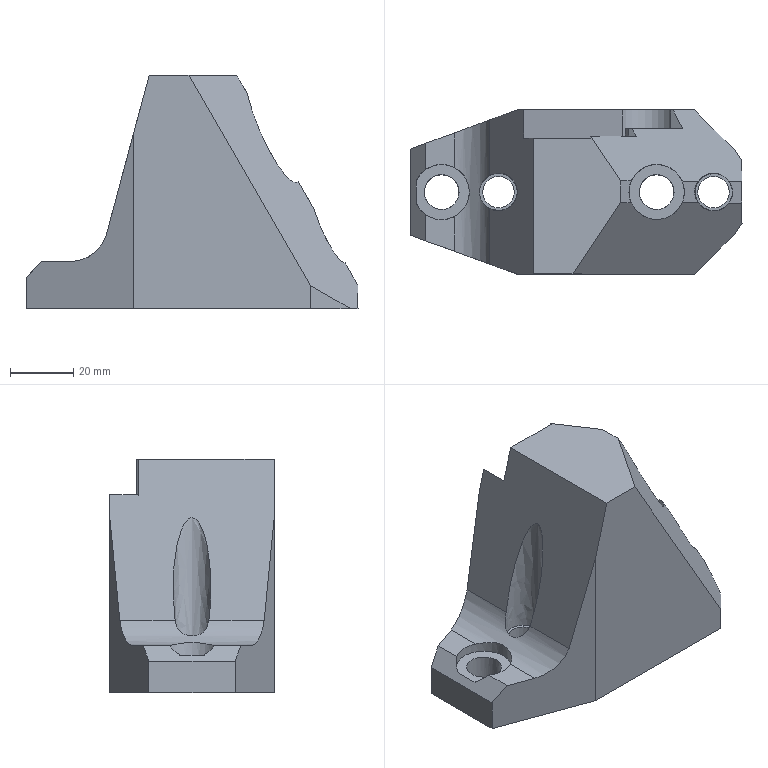Part | NX | features solid 2 | 1 solid | 41 faces | box 105 x 52 x 74 mm | volume 179080 mm3 | plane 30 | cylinder 8 | spline 3 | commonest cylinder face diameters 10 x2 11 x2 17.5 x1 17.501 x1 18.3 x1 24 x1
STEP:
#1=CARTESIAN_POINT('',(-407.032,-240.,159.));
#2=VERTEX_POINT('',#1);
#3=CARTESIAN_POINT('',(-407.032,-197.,159.));
#4=VERTEX_POINT('',#3);
#5=CARTESIAN_POINT('',(-407.032,-280.,159.));
#6=DIRECTION('',(0.,1.,0.));
#7=VECTOR('',#6,1000.);
#8=LINE('',#5,#7);
#9=EDGE_CURVE('',#2,#4,#8,.T.);
#10=ORIENTED_EDGE('',*,*,#9,.F.);
#11=CARTESIAN_POINT('',(-394.445,-240.,159.));
#12=VERTEX_POINT('',#11);
#13=CARTESIAN_POINT('',(-436.383,-240.,159.));
#14=DIRECTION('',(1.,0.,0.));
#15=VECTOR('',#14,1000.);
#16=LINE('',#13,#15);
#17=EDGE_CURVE('',#2,#12,#16,.T.);
#18=ORIENTED_EDGE('',*,*,#17,.T.);
#19=CARTESIAN_POINT('',(-379.421,-217.464,159.));
#20=VERTEX_POINT('',#19);
#21=CARTESIAN_POINT('',(-399.355,-247.365,159.));
#22=DIRECTION('',(0.5547,0.8321,0.));
#23=VECTOR('',#22,1000.);
#24=LINE('',#21,#23);
#25=EDGE_CURVE('',#12,#20,#24,.T.);
#26=ORIENTED_EDGE('',*,*,#25,.T.);
#27=CARTESIAN_POINT('',(-379.421,-210.536,159.));
#28=VERTEX_POINT('',#27);
#29=CARTESIAN_POINT('',(-379.421,-217.464,159.));
#30=DIRECTION('',(0.,1.,0.));
#31=VECTOR('',#30,1000.);
#32=LINE('',#29,#31);
#33=EDGE_CURVE('',#20,#28,#32,.T.);
#34=ORIENTED_EDGE('',*,*,#33,.T.);
#35=CARTESIAN_POINT('',(-388.839,-196.41,159.));
#36=VERTEX_POINT('',#35);
#37=CARTESIAN_POINT('',(-385.487,-201.438,159.));
#38=DIRECTION('',(-0.5547,0.8321,0.));
#39=VECTOR('',#38,1000.);
#40=LINE('',#37,#39);
#41=EDGE_CURVE('',#28,#36,#40,.T.);
#42=ORIENTED_EDGE('',*,*,#41,.T.);
#43=CARTESIAN_POINT('',(-388.839,-197.,159.));
#44=VERTEX_POINT('',#43);
#45=CARTESIAN_POINT('',(-388.839,-240.,159.));
#46=DIRECTION('',(0.,-1.,0.));
#47=VECTOR('',#46,1000.);
#48=LINE('',#45,#47);
#49=EDGE_CURVE('',#36,#44,#48,.T.);
#50=ORIENTED_EDGE('',*,*,#49,.T.);
#51=CARTESIAN_POINT('',(-407.032,-197.,159.));
#52=DIRECTION('',(-1.,0.,0.));
#53=VECTOR('',#52,1000.);
#54=LINE('',#51,#53);
#55=EDGE_CURVE('',#44,#4,#54,.T.);
#56=ORIENTED_EDGE('',*,*,#55,.T.);
#57=EDGE_LOOP('',(#10,#18,#26,#34,#42,#50,#56));
#58=FACE_BOUND('',#57,.T.);
#59=CARTESIAN_POINT('',(-407.032,-240.,159.));
#60=DIRECTION('',(0.,0.,1.));
#61=DIRECTION('',(0.,-1.,0.));
#62=AXIS2_PLACEMENT_3D('',#59,#60,#61);
#63=PLANE('',#62);
#64=ADVANCED_FACE('',(#58),#63,.T.);
#65=CARTESIAN_POINT('',(-432.,-195.279,100.002));
#66=VERTEX_POINT('',#65);
#67=CARTESIAN_POINT('',(-420.73,-191.177,107.88));
#68=VERTEX_POINT('',#67);
#69=CARTESIAN_POINT('',(-432.,-195.279,112.002));
#70=DIRECTION('',(0.342,-0.9397,0.));
#71=DIRECTION('',(0.9397,0.342,0.));
#72=AXIS2_PLACEMENT_3D('',#69,#70,#71);
#73=ELLIPSE('',#72,12.77,12.);
#74=EDGE_CURVE('',#66,#68,#73,.T.);
#75=ORIENTED_EDGE('',*,*,#74,.F.);
#76=CARTESIAN_POINT('',(-432.,-206.218,100.002));
#77=VERTEX_POINT('',#76);
#78=CARTESIAN_POINT('',(-432.,-280.,100.002));
#79=DIRECTION('',(0.,1.,0.));
#80=VECTOR('',#79,1000.);
#81=LINE('',#78,#80);
#82=EDGE_CURVE('',#77,#66,#81,.T.);
#83=ORIENTED_EDGE('',*,*,#82,.F.);
#84=CARTESIAN_POINT('',(-432.,-221.782,100.002));
#85=VERTEX_POINT('',#84);
#86=CARTESIAN_POINT('',(-432.,-206.218,100.002));
#87=CARTESIAN_POINT('',(-430.573,-206.951,100.002));
#88=CARTESIAN_POINT('',(-428.146,-209.212,100.538));
#89=CARTESIAN_POINT('',(-426.801,-214.004,101.205));
#90=CARTESIAN_POINT('',(-428.15,-218.796,100.536));
#91=CARTESIAN_POINT('',(-430.581,-221.053,100.002));
#92=CARTESIAN_POINT('',(-432.,-221.782,100.002));
#93=B_SPLINE_CURVE_WITH_KNOTS('',3,(#86,#87,#88,#89,#90,#91,#92),.UNSPECIFIED.,.F.,.F.,(4,1,1,1,4),(0.059,0.06377,0.06854,0.07331,0.07807),.UNSPECIFIED.);
#94=EDGE_CURVE('',#77,#85,#93,.T.);
#95=ORIENTED_EDGE('',*,*,#94,.T.);
#96=CARTESIAN_POINT('',(-432.,-232.721,100.002));
#97=VERTEX_POINT('',#96);
#98=CARTESIAN_POINT('',(-432.,-280.,100.002));
#99=DIRECTION('',(0.,1.,0.));
#100=VECTOR('',#99,1000.);
#101=LINE('',#98,#100);
#102=EDGE_CURVE('',#97,#85,#101,.T.);
#103=ORIENTED_EDGE('',*,*,#102,.F.);
#104=CARTESIAN_POINT('',(-420.73,-236.823,107.88));
#105=VERTEX_POINT('',#104);
#106=CARTESIAN_POINT('',(-432.,-232.721,112.002));
#107=DIRECTION('',(-0.342,-0.9397,0.));
#108=DIRECTION('',(-0.9397,0.342,0.));
#109=AXIS2_PLACEMENT_3D('',#106,#107,#108);
#110=ELLIPSE('',#109,12.77,12.);
#111=EDGE_CURVE('',#97,#105,#110,.T.);
#112=ORIENTED_EDGE('',*,*,#111,.T.);
#113=CARTESIAN_POINT('',(-420.73,-219.34,107.88));
#114=VERTEX_POINT('',#113);
#115=CARTESIAN_POINT('',(-420.73,-280.,107.88));
#116=DIRECTION('',(0.,1.,0.));
#117=VECTOR('',#116,1000.);
#118=LINE('',#115,#117);
#119=EDGE_CURVE('',#105,#114,#118,.T.);
#120=ORIENTED_EDGE('',*,*,#119,.T.);
#121=CARTESIAN_POINT('',(-420.73,-208.66,107.88));
#122=VERTEX_POINT('',#121);
#123=CARTESIAN_POINT('',(-420.73,-219.34,107.88));
#124=CARTESIAN_POINT('',(-420.975,-219.215,107.209));
#125=CARTESIAN_POINT('',(-421.568,-218.877,105.953));
#126=CARTESIAN_POINT('',(-422.701,-217.863,104.349));
#127=CARTESIAN_POINT('',(-423.711,-216.191,103.305));
#128=CARTESIAN_POINT('',(-424.14,-214.019,102.937));
#129=CARTESIAN_POINT('',(-423.728,-211.846,103.291));
#130=CARTESIAN_POINT('',(-422.369,-209.586,104.684));
#131=CARTESIAN_POINT('',(-421.223,-208.911,106.533));
#132=CARTESIAN_POINT('',(-420.73,-208.66,107.88));
#133=B_SPLINE_CURVE_WITH_KNOTS('',3,(#123,#124,#125,#126,#127,#128,#129,#130,#131,#132),.UNSPECIFIED.,.F.,.F.,(4,1,1,1,1,1,1,4),(0.,0.002143,0.004286,0.006429,0.008572,0.01071,0.01286,0.01714),.UNSPECIFIED.);
#134=EDGE_CURVE('',#114,#122,#133,.T.);
#135=ORIENTED_EDGE('',*,*,#134,.T.);
#136=CARTESIAN_POINT('',(-420.73,-280.,107.88));
#137=DIRECTION('',(0.,1.,0.));
#138=VECTOR('',#137,1000.);
#139=LINE('',#136,#138);
#140=EDGE_CURVE('',#122,#68,#139,.T.);
#141=ORIENTED_EDGE('',*,*,#140,.T.);
#142=EDGE_LOOP('',(#75,#83,#95,#103,#112,#120,#135,#141));
#143=FACE_BOUND('',#142,.T.);
#144=CARTESIAN_POINT('',(-432.,-280.,112.002));
#145=DIRECTION('',(0.,1.,0.));
#146=DIRECTION('',(0.,0.,1.));
#147=AXIS2_PLACEMENT_3D('',#144,#145,#146);
#148=CYLINDRICAL_SURFACE('',#147,12.);
#149=ADVANCED_FACE('',(#143),#148,.F.);
#150=CARTESIAN_POINT('',(-412.,-240.,140.46));
#151=VERTEX_POINT('',#150);
#152=CARTESIAN_POINT('',(-420.73,-240.,107.88));
#153=DIRECTION('',(-0.2588,0.,-0.9659));
#154=VECTOR('',#153,1000.);
#155=LINE('',#152,#154);
#156=EDGE_CURVE('',#2,#151,#155,.T.);
#157=ORIENTED_EDGE('',*,*,#156,.F.);
#158=ORIENTED_EDGE('',*,*,#9,.T.);
#159=CARTESIAN_POINT('',(-410.05,-197.,147.738));
#160=VERTEX_POINT('',#159);
#161=CARTESIAN_POINT('',(-420.73,-197.,107.88));
#162=DIRECTION('',(-0.2588,0.,-0.9659));
#163=VECTOR('',#162,1000.);
#164=LINE('',#161,#163);
#165=EDGE_CURVE('',#4,#160,#164,.T.);
#166=ORIENTED_EDGE('',*,*,#165,.T.);
#167=CARTESIAN_POINT('',(-410.05,-188.,147.738));
#168=VERTEX_POINT('',#167);
#169=CARTESIAN_POINT('',(-410.05,-197.,147.738));
#170=DIRECTION('',(0.,1.,0.));
#171=VECTOR('',#170,1000.);
#172=LINE('',#169,#171);
#173=EDGE_CURVE('',#168,#160,#172,.F.);
#174=ORIENTED_EDGE('',*,*,#173,.F.);
#175=CARTESIAN_POINT('',(-412.,-188.,140.46));
#176=VERTEX_POINT('',#175);
#177=CARTESIAN_POINT('',(-405.839,-188.,163.453));
#178=DIRECTION('',(0.2588,0.,0.9659));
#179=VECTOR('',#178,1000.);
#180=LINE('',#177,#179);
#181=EDGE_CURVE('',#176,#168,#180,.T.);
#182=ORIENTED_EDGE('',*,*,#181,.F.);
#183=CARTESIAN_POINT('',(-422.876,-191.959,99.869));
#184=DIRECTION('',(0.2577,0.09379,0.9617));
#185=VECTOR('',#184,1000.);
#186=LINE('',#183,#185);
#187=EDGE_CURVE('',#68,#176,#186,.T.);
#188=ORIENTED_EDGE('',*,*,#187,.F.);
#189=ORIENTED_EDGE('',*,*,#140,.F.);
#190=CARTESIAN_POINT('',(-420.73,-208.66,107.88));
#191=CARTESIAN_POINT('',(-419.967,-208.271,110.728));
#192=CARTESIAN_POINT('',(-418.819,-207.971,115.011));
#193=CARTESIAN_POINT('',(-417.281,-208.006,120.753));
#194=CARTESIAN_POINT('',(-416.131,-208.26,125.044));
#195=CARTESIAN_POINT('',(-414.988,-208.761,129.31));
#196=CARTESIAN_POINT('',(-414.04,-209.44,132.847));
#197=CARTESIAN_POINT('',(-413.301,-210.236,135.606));
#198=CARTESIAN_POINT('',(-412.759,-211.025,137.629));
#199=CARTESIAN_POINT('',(-412.336,-211.93,139.206));
#200=CARTESIAN_POINT('',(-412.057,-212.997,140.246));
#201=CARTESIAN_POINT('',(-411.963,-214.131,140.599));
#202=CARTESIAN_POINT('',(-412.098,-215.198,140.093));
#203=CARTESIAN_POINT('',(-412.388,-216.199,139.013));
#204=CARTESIAN_POINT('',(-412.817,-217.072,137.413));
#205=CARTESIAN_POINT('',(-413.355,-217.83,135.403));
#206=CARTESIAN_POINT('',(-414.098,-218.608,132.63));
#207=CARTESIAN_POINT('',(-415.032,-219.262,129.145));
#208=CARTESIAN_POINT('',(-416.164,-219.75,124.92));
#209=CARTESIAN_POINT('',(-417.303,-219.996,120.67));
#210=CARTESIAN_POINT('',(-418.832,-220.026,114.964));
#211=CARTESIAN_POINT('',(-419.972,-219.726,110.708));
#212=CARTESIAN_POINT('',(-420.73,-219.34,107.88));
#213=B_SPLINE_CURVE_WITH_KNOTS('',3,(#190,#191,#192,#193,#194,#195,#196,#197,#198,#199,#200,#201,#202,#203,#204,#205,#206,#207,#208,#209,#210,#211,#212),.UNSPECIFIED.,.F.,.F.,(4,1,1,1,1,1,1,1,1,1,1,1,1,1,1,1,1,1,1,1,4),(0.,0.008893,0.01334,0.01779,0.02223,0.02668,0.0289,0.03112,0.03335,0.03446,0.03557,0.03668,0.03779,0.04002,0.04224,0.04446,0.04891,0.05336,0.0578,0.06225,0.07114),.UNSPECIFIED.);
#214=EDGE_CURVE('',#122,#114,#213,.T.);
#215=ORIENTED_EDGE('',*,*,#214,.T.);
#216=ORIENTED_EDGE('',*,*,#119,.F.);
#217=CARTESIAN_POINT('',(-419.686,-237.202,111.774));
#218=DIRECTION('',(0.2577,-0.09379,0.9617));
#219=VECTOR('',#218,1000.);
#220=LINE('',#217,#219);
#221=EDGE_CURVE('',#105,#151,#220,.T.);
#222=ORIENTED_EDGE('',*,*,#221,.T.);
#223=EDGE_LOOP('',(#157,#158,#166,#174,#182,#188,#189,#215,#216,#222));
#224=FACE_BOUND('',#223,.T.);
#225=CARTESIAN_POINT('',(-420.73,-280.,107.88));
#226=DIRECTION('',(-0.9659,0.,0.2588));
#227=DIRECTION('',(0.2588,0.,0.9659));
#228=AXIS2_PLACEMENT_3D('',#225,#226,#227);
#229=PLANE('',#228);
#230=ADVANCED_FACE('',(#224),#229,.T.);
#231=CARTESIAN_POINT('',(-441.001,-229.445,100.002));
#232=VERTEX_POINT('',#231);
#233=CARTESIAN_POINT('',(-441.001,-221.181,100.002));
#234=VERTEX_POINT('',#233);
#235=CARTESIAN_POINT('',(-441.001,-280.,100.002));
#236=DIRECTION('',(0.,1.,0.));
#237=VECTOR('',#236,1000.);
#238=LINE('',#235,#237);
#239=EDGE_CURVE('',#232,#234,#238,.T.);
#240=ORIENTED_EDGE('',*,*,#239,.F.);
#241=CARTESIAN_POINT('',(-424.752,-235.359,100.002));
#242=DIRECTION('',(0.9397,-0.342,0.));
#243=VECTOR('',#242,1000.);
#244=LINE('',#241,#243);
#245=EDGE_CURVE('',#232,#97,#244,.T.);
#246=ORIENTED_EDGE('',*,*,#245,.T.);
#247=ORIENTED_EDGE('',*,*,#102,.T.);
#248=CARTESIAN_POINT('',(-436.,-214.,100.002));
#249=DIRECTION('',(0.,0.,1.));
#250=DIRECTION('',(1.,0.,0.));
#251=AXIS2_PLACEMENT_3D('',#248,#249,#250);
#252=CIRCLE('',#251,8.75);
#253=EDGE_CURVE('',#85,#234,#252,.F.);
#254=ORIENTED_EDGE('',*,*,#253,.T.);
#255=EDGE_LOOP('',(#240,#246,#247,#254));
#256=FACE_BOUND('',#255,.T.);
#257=CARTESIAN_POINT('',(-441.001,-280.,100.002));
#258=DIRECTION('',(0.,0.,1.));
#259=DIRECTION('',(1.,0.,0.));
#260=AXIS2_PLACEMENT_3D('',#257,#258,#259);
#261=PLANE('',#260);
#262=ADVANCED_FACE('',(#256),#261,.T.);
#263=CARTESIAN_POINT('',(-446.,-200.375,95.003));
#264=VERTEX_POINT('',#263);
#265=CARTESIAN_POINT('',(-441.001,-198.555,100.002));
#266=VERTEX_POINT('',#265);
#267=CARTESIAN_POINT('',(-459.59,-205.321,81.412));
#268=DIRECTION('',(0.6848,0.2492,0.6848));
#269=VECTOR('',#268,1000.);
#270=LINE('',#267,#269);
#271=EDGE_CURVE('',#264,#266,#270,.T.);
#272=ORIENTED_EDGE('',*,*,#271,.F.);
#273=CARTESIAN_POINT('',(-446.,-227.625,95.003));
#274=VERTEX_POINT('',#273);
#275=CARTESIAN_POINT('',(-446.,-280.,95.003));
#276=DIRECTION('',(0.,1.,0.));
#277=VECTOR('',#276,1000.);
#278=LINE('',#275,#277);
#279=EDGE_CURVE('',#274,#264,#278,.T.);
#280=ORIENTED_EDGE('',*,*,#279,.F.);
#281=CARTESIAN_POINT('',(-437.061,-230.879,103.942));
#282=DIRECTION('',(0.6848,-0.2492,0.6848));
#283=VECTOR('',#282,1000.);
#284=LINE('',#281,#283);
#285=EDGE_CURVE('',#274,#232,#284,.T.);
#286=ORIENTED_EDGE('',*,*,#285,.T.);
#287=ORIENTED_EDGE('',*,*,#239,.T.);
#288=CARTESIAN_POINT('',(-444.001,-217.544,97.002));
#289=VERTEX_POINT('',#288);
#290=CARTESIAN_POINT('',(-436.,-214.,105.003));
#291=DIRECTION('',(-0.7071,0.,0.7071));
#292=DIRECTION('',(-0.7071,0.,-0.7071));
#293=AXIS2_PLACEMENT_3D('',#290,#291,#292);
#294=ELLIPSE('',#293,12.375,8.75);
#295=EDGE_CURVE('',#234,#289,#294,.F.);
#296=ORIENTED_EDGE('',*,*,#295,.T.);
#297=CARTESIAN_POINT('',(-444.001,-210.456,97.002));
#298=VERTEX_POINT('',#297);
#299=CARTESIAN_POINT('',(-444.001,-280.,97.002));
#300=DIRECTION('',(0.,1.,0.));
#301=VECTOR('',#300,1000.);
#302=LINE('',#299,#301);
#303=EDGE_CURVE('',#289,#298,#302,.T.);
#304=ORIENTED_EDGE('',*,*,#303,.T.);
#305=CARTESIAN_POINT('',(-441.001,-206.819,100.002));
#306=VERTEX_POINT('',#305);
#307=CARTESIAN_POINT('',(-436.,-214.,105.003));
#308=DIRECTION('',(-0.7071,0.,0.7071));
#309=DIRECTION('',(-0.7071,0.,-0.7071));
#310=AXIS2_PLACEMENT_3D('',#307,#308,#309);
#311=ELLIPSE('',#310,12.375,8.75);
#312=EDGE_CURVE('',#298,#306,#311,.F.);
#313=ORIENTED_EDGE('',*,*,#312,.T.);
#314=CARTESIAN_POINT('',(-441.001,-280.,100.002));
#315=DIRECTION('',(0.,1.,0.));
#316=VECTOR('',#315,1000.);
#317=LINE('',#314,#316);
#318=EDGE_CURVE('',#306,#266,#317,.T.);
#319=ORIENTED_EDGE('',*,*,#318,.T.);
#320=EDGE_LOOP('',(#272,#280,#286,#287,#296,#304,#313,#319));
#321=FACE_BOUND('',#320,.T.);
#322=CARTESIAN_POINT('',(-446.,-280.,95.003));
#323=DIRECTION('',(-0.7071,0.,0.7071));
#324=DIRECTION('',(0.7071,0.,0.7071));
#325=AXIS2_PLACEMENT_3D('',#322,#323,#324);
#326=PLANE('',#325);
#327=ADVANCED_FACE('',(#321),#326,.T.);
#328=CARTESIAN_POINT('',(-436.,-219.5,85.));
#329=VERTEX_POINT('',#328);
#330=CARTESIAN_POINT('',(-436.,-214.,85.));
#331=DIRECTION('',(0.,0.,1.));
#332=DIRECTION('',(0.,-1.,0.));
#333=AXIS2_PLACEMENT_3D('',#330,#331,#332);
#334=CIRCLE('',#333,5.5);
#335=EDGE_CURVE('',#329,#329,#334,.T.);
#336=ORIENTED_EDGE('',*,*,#335,.T.);
#337=EDGE_LOOP('',(#336));
#338=FACE_BOUND('',#337,.T.);
#339=CARTESIAN_POINT('',(-368.,-219.5,85.));
#340=VERTEX_POINT('',#339);
#341=CARTESIAN_POINT('',(-368.,-214.,85.));
#342=DIRECTION('',(0.,0.,1.));
#343=DIRECTION('',(0.,-1.,0.));
#344=AXIS2_PLACEMENT_3D('',#341,#342,#343);
#345=CIRCLE('',#344,5.5);
#346=EDGE_CURVE('',#340,#340,#345,.T.);
#347=ORIENTED_EDGE('',*,*,#346,.T.);
#348=EDGE_LOOP('',(#347));
#349=FACE_BOUND('',#348,.T.);
#350=CARTESIAN_POINT('',(-350.,-219.,85.));
#351=VERTEX_POINT('',#350);
#352=CARTESIAN_POINT('',(-350.,-214.,85.));
#353=DIRECTION('',(0.,0.,1.));
#354=DIRECTION('',(0.,-1.,0.));
#355=AXIS2_PLACEMENT_3D('',#352,#353,#354);
#356=CIRCLE('',#355,5.);
#357=EDGE_CURVE('',#351,#351,#356,.T.);
#358=ORIENTED_EDGE('',*,*,#357,.T.);
#359=EDGE_LOOP('',(#358));
#360=FACE_BOUND('',#359,.T.);
#361=CARTESIAN_POINT('',(-418.,-219.,85.));
#362=VERTEX_POINT('',#361);
#363=CARTESIAN_POINT('',(-418.,-214.,85.));
#364=DIRECTION('',(0.,0.,1.));
#365=DIRECTION('',(0.,-1.,0.));
#366=AXIS2_PLACEMENT_3D('',#363,#364,#365);
#367=CIRCLE('',#366,5.);
#368=EDGE_CURVE('',#362,#362,#367,.T.);
#369=ORIENTED_EDGE('',*,*,#368,.T.);
#370=EDGE_LOOP('',(#369));
#371=FACE_BOUND('',#370,.T.);
#372=CARTESIAN_POINT('',(-341.,-204.082,85.));
#373=VERTEX_POINT('',#372);
#374=CARTESIAN_POINT('',(-341.,-223.918,85.));
#375=VERTEX_POINT('',#374);
#376=CARTESIAN_POINT('',(-341.,-240.,85.));
#377=DIRECTION('',(0.,-1.,0.));
#378=VECTOR('',#377,1000.);
#379=LINE('',#376,#378);
#380=EDGE_CURVE('',#373,#375,#379,.T.);
#381=ORIENTED_EDGE('',*,*,#380,.T.);
#382=CARTESIAN_POINT('',(-343.164,-227.164,85.));
#383=VERTEX_POINT('',#382);
#384=CARTESIAN_POINT('',(-380.73,-283.513,85.));
#385=DIRECTION('',(-0.5547,-0.8321,0.));
#386=VECTOR('',#385,1000.);
#387=LINE('',#384,#386);
#388=EDGE_CURVE('',#375,#383,#387,.T.);
#389=ORIENTED_EDGE('',*,*,#388,.T.);
#390=CARTESIAN_POINT('',(-356.,-240.,85.));
#391=VERTEX_POINT('',#390);
#392=CARTESIAN_POINT('',(-341.,-225.,85.));
#393=DIRECTION('',(-0.7071,-0.7071,0.));
#394=VECTOR('',#393,1000.);
#395=LINE('',#392,#394);
#396=EDGE_CURVE('',#383,#391,#395,.T.);
#397=ORIENTED_EDGE('',*,*,#396,.T.);
#398=CARTESIAN_POINT('',(-412.,-240.,85.));
#399=VERTEX_POINT('',#398);
#400=CARTESIAN_POINT('',(-436.383,-240.,85.));
#401=DIRECTION('',(1.,0.,0.));
#402=VECTOR('',#401,1000.);
#403=LINE('',#400,#402);
#404=EDGE_CURVE('',#399,#391,#403,.T.);
#405=ORIENTED_EDGE('',*,*,#404,.F.);
#406=CARTESIAN_POINT('',(-446.,-227.625,85.));
#407=VERTEX_POINT('',#406);
#408=CARTESIAN_POINT('',(-442.023,-229.073,85.));
#409=DIRECTION('',(0.9397,-0.342,0.));
#410=VECTOR('',#409,1000.);
#411=LINE('',#408,#410);
#412=EDGE_CURVE('',#407,#399,#411,.T.);
#413=ORIENTED_EDGE('',*,*,#412,.F.);
#414=CARTESIAN_POINT('',(-446.,-200.375,85.));
#415=VERTEX_POINT('',#414);
#416=CARTESIAN_POINT('',(-446.,-240.,85.));
#417=DIRECTION('',(0.,-1.,0.));
#418=VECTOR('',#417,1000.);
#419=LINE('',#416,#418);
#420=EDGE_CURVE('',#415,#407,#419,.T.);
#421=ORIENTED_EDGE('',*,*,#420,.F.);
#422=CARTESIAN_POINT('',(-412.,-188.,85.));
#423=VERTEX_POINT('',#422);
#424=CARTESIAN_POINT('',(-458.735,-205.01,85.));
#425=DIRECTION('',(0.9397,0.342,0.));
#426=VECTOR('',#425,1000.);
#427=LINE('',#424,#426);
#428=EDGE_CURVE('',#415,#423,#427,.T.);
#429=ORIENTED_EDGE('',*,*,#428,.T.);
#430=CARTESIAN_POINT('',(-356.,-188.,85.));
#431=VERTEX_POINT('',#430);
#432=CARTESIAN_POINT('',(-436.383,-188.,85.));
#433=DIRECTION('',(1.,0.,0.));
#434=VECTOR('',#433,1000.);
#435=LINE('',#432,#434);
#436=EDGE_CURVE('',#423,#431,#435,.T.);
#437=ORIENTED_EDGE('',*,*,#436,.T.);
#438=CARTESIAN_POINT('',(-343.164,-200.836,85.));
#439=VERTEX_POINT('',#438);
#440=CARTESIAN_POINT('',(-356.,-188.,85.));
#441=DIRECTION('',(-0.7071,0.7071,0.));
#442=VECTOR('',#441,1000.);
#443=LINE('',#440,#442);
#444=EDGE_CURVE('',#431,#439,#443,.F.);
#445=ORIENTED_EDGE('',*,*,#444,.T.);
#446=CARTESIAN_POINT('',(-356.73,-180.487,85.));
#447=DIRECTION('',(0.5547,-0.8321,0.));
#448=VECTOR('',#447,1000.);
#449=LINE('',#446,#448);
#450=EDGE_CURVE('',#439,#373,#449,.T.);
#451=ORIENTED_EDGE('',*,*,#450,.T.);
#452=EDGE_LOOP('',(#381,#389,#397,#405,#413,#421,#429,#437,#445,#451));
#453=FACE_BOUND('',#452,.T.);
#454=CARTESIAN_POINT('',(-446.,-240.,85.));
#455=DIRECTION('',(0.,0.,1.));
#456=DIRECTION('',(0.,-1.,0.));
#457=AXIS2_PLACEMENT_3D('',#454,#455,#456);
#458=PLANE('',#457);
#459=ADVANCED_FACE('',(#338,#349,#360,#371,#453),#458,.F.);
#460=ORIENTED_EDGE('',*,*,#17,.F.);
#461=ORIENTED_EDGE('',*,*,#156,.T.);
#462=CARTESIAN_POINT('',(-412.,-240.,171.637));
#463=DIRECTION('',(0.,0.,1.));
#464=VECTOR('',#463,1000.);
#465=LINE('',#462,#464);
#466=EDGE_CURVE('',#399,#151,#465,.T.);
#467=ORIENTED_EDGE('',*,*,#466,.F.);
#468=ORIENTED_EDGE('',*,*,#404,.T.);
#469=CARTESIAN_POINT('',(-356.,-240.,92.411));
#470=VERTEX_POINT('',#469);
#471=CARTESIAN_POINT('',(-356.,-240.,92.452));
#472=DIRECTION('',(0.,0.,1.));
#473=VECTOR('',#472,1000.);
#474=LINE('',#471,#473);
#475=EDGE_CURVE('',#391,#470,#474,.T.);
#476=ORIENTED_EDGE('',*,*,#475,.T.);
#477=CARTESIAN_POINT('',(-410.402,-240.,186.637));
#478=DIRECTION('',(0.5,0.,-0.866));
#479=VECTOR('',#478,1000.);
#480=LINE('',#477,#479);
#481=EDGE_CURVE('',#12,#470,#480,.T.);
#482=ORIENTED_EDGE('',*,*,#481,.F.);
#483=EDGE_LOOP('',(#460,#461,#467,#468,#476,#482));
#484=FACE_BOUND('',#483,.T.);
#485=CARTESIAN_POINT('',(-436.383,-240.,171.637));
#486=DIRECTION('',(0.,1.,0.));
#487=DIRECTION('',(-1.,0.,0.));
#488=AXIS2_PLACEMENT_3D('',#485,#486,#487);
#489=PLANE('',#488);
#490=ADVANCED_FACE('',(#484),#489,.F.);
#491=ORIENTED_EDGE('',*,*,#279,.T.);
#492=CARTESIAN_POINT('',(-446.,-200.375,95.003));
#493=DIRECTION('',(0.,0.,-1.));
#494=VECTOR('',#493,1000.);
#495=LINE('',#492,#494);
#496=EDGE_CURVE('',#264,#415,#495,.T.);
#497=ORIENTED_EDGE('',*,*,#496,.T.);
#498=ORIENTED_EDGE('',*,*,#420,.T.);
#499=CARTESIAN_POINT('',(-446.,-227.625,95.003));
#500=DIRECTION('',(0.,0.,-1.));
#501=VECTOR('',#500,1000.);
#502=LINE('',#499,#501);
#503=EDGE_CURVE('',#274,#407,#502,.T.);
#504=ORIENTED_EDGE('',*,*,#503,.F.);
#505=EDGE_LOOP('',(#491,#497,#498,#504));
#506=FACE_BOUND('',#505,.T.);
#507=CARTESIAN_POINT('',(-446.,-240.,95.003));
#508=DIRECTION('',(1.,0.,0.));
#509=DIRECTION('',(0.,1.,0.));
#510=AXIS2_PLACEMENT_3D('',#507,#508,#509);
#511=PLANE('',#510);
#512=ADVANCED_FACE('',(#506),#511,.F.);
#513=ORIENTED_EDGE('',*,*,#450,.F.);
#514=CARTESIAN_POINT('',(-356.,-188.,92.411));
#515=VERTEX_POINT('',#514);
#516=CARTESIAN_POINT('',(-375.604,-168.396,103.729));
#517=DIRECTION('',(0.6547,-0.6547,-0.378));
#518=VECTOR('',#517,1000.);
#519=LINE('',#516,#518);
#520=EDGE_CURVE('',#439,#515,#519,.F.);
#521=ORIENTED_EDGE('',*,*,#520,.T.);
#522=CARTESIAN_POINT('',(-362.787,-188.,104.166));
#523=VERTEX_POINT('',#522);
#524=CARTESIAN_POINT('',(-410.402,-188.,186.637));
#525=DIRECTION('',(0.5,0.,-0.866));
#526=VECTOR('',#525,1000.);
#527=LINE('',#524,#526);
#528=EDGE_CURVE('',#523,#515,#527,.T.);
#529=ORIENTED_EDGE('',*,*,#528,.F.);
#530=CARTESIAN_POINT('',(-359.787,-194.,105.898));
#531=VERTEX_POINT('',#530);
#532=CARTESIAN_POINT('',(-351.519,-210.536,110.671));
#533=DIRECTION('',(0.433,-0.866,0.25));
#534=VECTOR('',#533,1000.);
#535=LINE('',#532,#534);
#536=EDGE_CURVE('',#523,#531,#535,.T.);
#537=ORIENTED_EDGE('',*,*,#536,.T.);
#538=CARTESIAN_POINT('',(-375.684,-194.,133.433));
#539=VERTEX_POINT('',#538);
#540=CARTESIAN_POINT('',(-407.402,-194.,188.37));
#541=DIRECTION('',(0.5,0.,-0.866));
#542=VECTOR('',#541,1000.);
#543=LINE('',#540,#542);
#544=EDGE_CURVE('',#539,#531,#543,.T.);
#545=ORIENTED_EDGE('',*,*,#544,.F.);
#546=CARTESIAN_POINT('',(-374.48,-196.41,134.129));
#547=VERTEX_POINT('',#546);
#548=CARTESIAN_POINT('',(-367.416,-210.536,138.207));
#549=DIRECTION('',(0.433,-0.866,0.25));
#550=VECTOR('',#549,1000.);
#551=LINE('',#548,#550);
#552=EDGE_CURVE('',#539,#547,#551,.T.);
#553=ORIENTED_EDGE('',*,*,#552,.T.);
#554=CARTESIAN_POINT('',(-406.197,-196.41,189.065));
#555=DIRECTION('',(0.5,0.,-0.866));
#556=VECTOR('',#555,1000.);
#557=LINE('',#554,#556);
#558=EDGE_CURVE('',#36,#547,#557,.T.);
#559=ORIENTED_EDGE('',*,*,#558,.F.);
#560=ORIENTED_EDGE('',*,*,#41,.F.);
#561=CARTESIAN_POINT('',(-376.035,-210.536,153.135));
#562=VERTEX_POINT('',#561);
#563=CARTESIAN_POINT('',(-399.134,-210.536,193.143));
#564=DIRECTION('',(0.5,0.,-0.866));
#565=VECTOR('',#564,1000.);
#566=LINE('',#563,#565);
#567=EDGE_CURVE('',#28,#562,#566,.T.);
#568=ORIENTED_EDGE('',*,*,#567,.T.);
#569=CARTESIAN_POINT('',(-359.965,-210.536,125.3));
#570=VERTEX_POINT('',#569);
#571=CARTESIAN_POINT('',(-368.,-214.,143.217));
#572=DIRECTION('',(-0.75,-0.5,-0.433));
#573=DIRECTION('',(0.3603,0.2402,-0.9014));
#574=AXIS2_PLACEMENT_3D('',#571,#572,#573);
#575=ELLIPSE('',#574,20.207,8.75);
#576=EDGE_CURVE('',#570,#562,#575,.F.);
#577=ORIENTED_EDGE('',*,*,#576,.F.);
#578=CARTESIAN_POINT('',(-354.897,-210.536,116.523));
#579=VERTEX_POINT('',#578);
#580=CARTESIAN_POINT('',(-399.134,-210.536,193.143));
#581=DIRECTION('',(0.5,0.,-0.866));
#582=VECTOR('',#581,1000.);
#583=LINE('',#580,#582);
#584=EDGE_CURVE('',#570,#579,#583,.T.);
#585=ORIENTED_EDGE('',*,*,#584,.T.);
#586=CARTESIAN_POINT('',(-345.103,-210.536,99.558));
#587=VERTEX_POINT('',#586);
#588=CARTESIAN_POINT('',(-345.103,-210.536,99.558));
#589=CARTESIAN_POINT('',(-345.612,-209.813,99.605));
#590=CARTESIAN_POINT('',(-346.862,-208.755,100.55));
#591=CARTESIAN_POINT('',(-348.449,-208.146,102.594));
#592=CARTESIAN_POINT('',(-349.855,-207.95,104.804));
#593=CARTESIAN_POINT('',(-351.54,-208.106,107.902));
#594=CARTESIAN_POINT('',(-353.308,-208.834,111.804));
#595=CARTESIAN_POINT('',(-354.434,-209.879,114.962));
#596=CARTESIAN_POINT('',(-354.897,-210.536,116.523));
#597=B_SPLINE_CURVE_WITH_KNOTS('',3,(#588,#589,#590,#591,#592,#593,#594,#595,#596),.UNSPECIFIED.,.F.,.F.,(4,1,1,1,1,1,4),(0.002898,0.005552,0.008207,0.01086,0.01352,0.01883,0.02413),.UNSPECIFIED.);
#598=EDGE_CURVE('',#587,#579,#597,.T.);
#599=ORIENTED_EDGE('',*,*,#598,.F.);
#600=CARTESIAN_POINT('',(-341.,-210.536,92.452));
#601=VERTEX_POINT('',#600);
#602=CARTESIAN_POINT('',(-399.134,-210.536,193.143));
#603=DIRECTION('',(0.5,0.,-0.866));
#604=VECTOR('',#603,1000.);
#605=LINE('',#602,#604);
#606=EDGE_CURVE('',#587,#601,#605,.T.);
#607=ORIENTED_EDGE('',*,*,#606,.T.);
#608=CARTESIAN_POINT('',(-341.,-260.365,149.99));
#609=DIRECTION('',(0.,-0.6547,0.7559));
#610=VECTOR('',#609,1000.);
#611=LINE('',#608,#610);
#612=EDGE_CURVE('',#373,#601,#611,.T.);
#613=ORIENTED_EDGE('',*,*,#612,.F.);
#614=EDGE_LOOP('',(#513,#521,#529,#537,#545,#553,#559,#560,#568,#577,#585,#599,#607,#613));
#615=FACE_BOUND('',#614,.T.);
#616=CARTESIAN_POINT('',(-399.134,-210.536,193.143));
#617=DIRECTION('',(-0.75,-0.5,-0.433));
#618=DIRECTION('',(0.5547,-0.8321,0.));
#619=AXIS2_PLACEMENT_3D('',#616,#617,#618);
#620=PLANE('',#619);
#621=ADVANCED_FACE('',(#615),#620,.F.);
#622=CARTESIAN_POINT('',(-354.897,-217.464,116.523));
#623=VERTEX_POINT('',#622);
#624=CARTESIAN_POINT('',(-354.897,-210.536,116.523));
#625=CARTESIAN_POINT('',(-355.188,-210.949,117.027));
#626=CARTESIAN_POINT('',(-355.724,-211.904,117.954));
#627=CARTESIAN_POINT('',(-356.139,-214.006,118.674));
#628=CARTESIAN_POINT('',(-355.72,-216.103,117.948));
#629=CARTESIAN_POINT('',(-355.188,-217.051,117.026));
#630=CARTESIAN_POINT('',(-354.897,-217.464,116.523));
#631=B_SPLINE_CURVE_WITH_KNOTS('',3,(#624,#625,#626,#627,#628,#629,#630),.UNSPECIFIED.,.F.,.F.,(4,1,1,1,4),(0.,0.002127,0.004253,0.00638,0.008507),.UNSPECIFIED.);
#632=EDGE_CURVE('',#579,#623,#631,.T.);
#633=ORIENTED_EDGE('',*,*,#632,.F.);
#634=ORIENTED_EDGE('',*,*,#584,.F.);
#635=CARTESIAN_POINT('',(-359.965,-217.464,125.3));
#636=VERTEX_POINT('',#635);
#637=CARTESIAN_POINT('',(-368.,-214.,139.217));
#638=DIRECTION('',(-0.866,0.,-0.5));
#639=DIRECTION('',(0.5,0.,-0.866));
#640=AXIS2_PLACEMENT_3D('',#637,#638,#639);
#641=ELLIPSE('',#640,17.5,8.75);
#642=EDGE_CURVE('',#636,#570,#641,.F.);
#643=ORIENTED_EDGE('',*,*,#642,.F.);
#644=CARTESIAN_POINT('',(-399.134,-217.464,193.143));
#645=DIRECTION('',(0.5,0.,-0.866));
#646=VECTOR('',#645,1000.);
#647=LINE('',#644,#646);
#648=EDGE_CURVE('',#636,#623,#647,.T.);
#649=ORIENTED_EDGE('',*,*,#648,.T.);
#650=EDGE_LOOP('',(#633,#634,#643,#649));
#651=FACE_BOUND('',#650,.T.);
#652=CARTESIAN_POINT('',(-399.134,-217.464,193.143));
#653=DIRECTION('',(-0.866,0.,-0.5));
#654=DIRECTION('',(-0.5,0.,0.866));
#655=AXIS2_PLACEMENT_3D('',#652,#653,#654);
#656=PLANE('',#655);
#657=ADVANCED_FACE('',(#651),#656,.F.);
#658=ORIENTED_EDGE('',*,*,#388,.F.);
#659=CARTESIAN_POINT('',(-341.,-217.464,92.452));
#660=VERTEX_POINT('',#659);
#661=CARTESIAN_POINT('',(-341.,-180.513,135.12));
#662=DIRECTION('',(0.,-0.6547,-0.7559));
#663=VECTOR('',#662,1000.);
#664=LINE('',#661,#663);
#665=EDGE_CURVE('',#660,#375,#664,.T.);
#666=ORIENTED_EDGE('',*,*,#665,.F.);
#667=CARTESIAN_POINT('',(-345.103,-217.464,99.558));
#668=VERTEX_POINT('',#667);
#669=CARTESIAN_POINT('',(-399.134,-217.464,193.143));
#670=DIRECTION('',(0.5,0.,-0.866));
#671=VECTOR('',#670,1000.);
#672=LINE('',#669,#671);
#673=EDGE_CURVE('',#668,#660,#672,.T.);
#674=ORIENTED_EDGE('',*,*,#673,.F.);
#675=CARTESIAN_POINT('',(-354.897,-217.464,116.523));
#676=CARTESIAN_POINT('',(-354.433,-218.123,114.958));
#677=CARTESIAN_POINT('',(-353.319,-219.158,111.833));
#678=CARTESIAN_POINT('',(-351.537,-219.895,107.895));
#679=CARTESIAN_POINT('',(-349.855,-220.05,104.804));
#680=CARTESIAN_POINT('',(-348.44,-219.852,102.582));
#681=CARTESIAN_POINT('',(-346.868,-219.248,100.555));
#682=CARTESIAN_POINT('',(-345.61,-218.185,99.605));
#683=CARTESIAN_POINT('',(-345.103,-217.464,99.558));
#684=B_SPLINE_CURVE_WITH_KNOTS('',3,(#675,#676,#677,#678,#679,#680,#681,#682,#683),.UNSPECIFIED.,.F.,.F.,(4,1,1,1,1,1,4),(0.01401,0.01933,0.02464,0.0273,0.02996,0.03261,0.03527),.UNSPECIFIED.);
#685=EDGE_CURVE('',#623,#668,#684,.T.);
#686=ORIENTED_EDGE('',*,*,#685,.F.);
#687=ORIENTED_EDGE('',*,*,#648,.F.);
#688=CARTESIAN_POINT('',(-376.035,-217.464,153.135));
#689=VERTEX_POINT('',#688);
#690=CARTESIAN_POINT('',(-368.,-214.,143.217));
#691=DIRECTION('',(-0.75,0.5,-0.433));
#692=DIRECTION('',(0.3603,-0.2402,-0.9014));
#693=AXIS2_PLACEMENT_3D('',#690,#691,#692);
#694=ELLIPSE('',#693,20.207,8.75);
#695=EDGE_CURVE('',#689,#636,#694,.F.);
#696=ORIENTED_EDGE('',*,*,#695,.F.);
#697=CARTESIAN_POINT('',(-399.134,-217.464,193.143));
#698=DIRECTION('',(0.5,0.,-0.866));
#699=VECTOR('',#698,1000.);
#700=LINE('',#697,#699);
#701=EDGE_CURVE('',#20,#689,#700,.T.);
#702=ORIENTED_EDGE('',*,*,#701,.F.);
#703=ORIENTED_EDGE('',*,*,#25,.F.);
#704=ORIENTED_EDGE('',*,*,#481,.T.);
#705=CARTESIAN_POINT('',(-343.153,-227.153,84.993));
#706=DIRECTION('',(0.6547,0.6547,-0.378));
#707=VECTOR('',#706,1000.);
#708=LINE('',#705,#707);
#709=EDGE_CURVE('',#470,#383,#708,.T.);
#710=ORIENTED_EDGE('',*,*,#709,.T.);
#711=EDGE_LOOP('',(#658,#666,#674,#686,#687,#696,#702,#703,#704,#710));
#712=FACE_BOUND('',#711,.T.);
#713=CARTESIAN_POINT('',(-410.402,-240.,186.637));
#714=DIRECTION('',(-0.75,0.5,-0.433));
#715=DIRECTION('',(-0.5547,-0.8321,0.));
#716=AXIS2_PLACEMENT_3D('',#713,#714,#715);
#717=PLANE('',#716);
#718=ADVANCED_FACE('',(#712),#717,.F.);
#719=CARTESIAN_POINT('',(-345.103,-217.464,99.558));
#720=CARTESIAN_POINT('',(-344.812,-217.051,99.054));
#721=CARTESIAN_POINT('',(-344.276,-216.096,98.127));
#722=CARTESIAN_POINT('',(-343.861,-213.994,97.407));
#723=CARTESIAN_POINT('',(-344.28,-211.897,98.133));
#724=CARTESIAN_POINT('',(-344.812,-210.949,99.055));
#725=CARTESIAN_POINT('',(-345.103,-210.536,99.558));
#726=B_SPLINE_CURVE_WITH_KNOTS('',3,(#719,#720,#721,#722,#723,#724,#725),.UNSPECIFIED.,.F.,.F.,(4,1,1,1,4),(0.,0.002127,0.004253,0.00638,0.008507),.UNSPECIFIED.);
#727=EDGE_CURVE('',#668,#587,#726,.T.);
#728=ORIENTED_EDGE('',*,*,#727,.F.);
#729=ORIENTED_EDGE('',*,*,#673,.T.);
#730=CARTESIAN_POINT('',(-341.,-217.464,92.452));
#731=DIRECTION('',(0.,-1.,0.));
#732=VECTOR('',#731,1000.);
#733=LINE('',#730,#732);
#734=EDGE_CURVE('',#601,#660,#733,.T.);
#735=ORIENTED_EDGE('',*,*,#734,.F.);
#736=ORIENTED_EDGE('',*,*,#606,.F.);
#737=EDGE_LOOP('',(#728,#729,#735,#736));
#738=FACE_BOUND('',#737,.T.);
#739=CARTESIAN_POINT('',(-399.134,-217.464,193.143));
#740=DIRECTION('',(-0.866,0.,-0.5));
#741=DIRECTION('',(-0.5,0.,0.866));
#742=AXIS2_PLACEMENT_3D('',#739,#740,#741);
#743=PLANE('',#742);
#744=ADVANCED_FACE('',(#738),#743,.F.);
#745=CARTESIAN_POINT('',(-467.176,-208.083,100.002));
#746=DIRECTION('',(0.9397,0.342,0.));
#747=VECTOR('',#746,1000.);
#748=LINE('',#745,#747);
#749=EDGE_CURVE('',#266,#66,#748,.T.);
#750=ORIENTED_EDGE('',*,*,#749,.F.);
#751=ORIENTED_EDGE('',*,*,#318,.F.);
#752=CARTESIAN_POINT('',(-436.,-214.,100.002));
#753=DIRECTION('',(0.,0.,1.));
#754=DIRECTION('',(1.,0.,0.));
#755=AXIS2_PLACEMENT_3D('',#752,#753,#754);
#756=CIRCLE('',#755,8.75);
#757=EDGE_CURVE('',#306,#77,#756,.F.);
#758=ORIENTED_EDGE('',*,*,#757,.T.);
#759=ORIENTED_EDGE('',*,*,#82,.T.);
#760=EDGE_LOOP('',(#750,#751,#758,#759));
#761=FACE_BOUND('',#760,.T.);
#762=CARTESIAN_POINT('',(-441.001,-280.,100.002));
#763=DIRECTION('',(0.,0.,1.));
#764=DIRECTION('',(1.,0.,0.));
#765=AXIS2_PLACEMENT_3D('',#762,#763,#764);
#766=PLANE('',#765);
#767=ADVANCED_FACE('',(#761),#766,.T.);
#768=ORIENTED_EDGE('',*,*,#335,.F.);
#769=EDGE_LOOP('',(#768));
#770=FACE_BOUND('',#769,.T.);
#771=CARTESIAN_POINT('',(-430.5,-214.,97.002));
#772=VERTEX_POINT('',#771);
#773=CARTESIAN_POINT('',(-436.,-214.,97.002));
#774=DIRECTION('',(0.,0.,1.));
#775=DIRECTION('',(1.,0.,0.));
#776=AXIS2_PLACEMENT_3D('',#773,#774,#775);
#777=CIRCLE('',#776,5.5);
#778=EDGE_CURVE('',#772,#772,#777,.T.);
#779=ORIENTED_EDGE('',*,*,#778,.T.);
#780=EDGE_LOOP('',(#779));
#781=FACE_BOUND('',#780,.T.);
#782=CARTESIAN_POINT('',(-436.,-214.,205.002));
#783=DIRECTION('',(0.,0.,-1.));
#784=DIRECTION('',(-1.,0.,0.));
#785=AXIS2_PLACEMENT_3D('',#782,#783,#784);
#786=CYLINDRICAL_SURFACE('',#785,5.5);
#787=ADVANCED_FACE('',(#770,#781),#786,.F.);
#788=CARTESIAN_POINT('',(-368.,-214.,139.217));
#789=DIRECTION('',(-0.866,0.,-0.5));
#790=DIRECTION('',(0.5,0.,-0.866));
#791=AXIS2_PLACEMENT_3D('',#788,#789,#790);
#792=ELLIPSE('',#791,17.5,8.75);
#793=EDGE_CURVE('',#562,#689,#792,.F.);
#794=ORIENTED_EDGE('',*,*,#793,.F.);
#795=ORIENTED_EDGE('',*,*,#567,.F.);
#796=ORIENTED_EDGE('',*,*,#33,.F.);
#797=ORIENTED_EDGE('',*,*,#701,.T.);
#798=EDGE_LOOP('',(#794,#795,#796,#797));
#799=FACE_BOUND('',#798,.T.);
#800=CARTESIAN_POINT('',(-399.134,-217.464,193.143));
#801=DIRECTION('',(-0.866,0.,-0.5));
#802=DIRECTION('',(-0.5,0.,0.866));
#803=AXIS2_PLACEMENT_3D('',#800,#801,#802);
#804=PLANE('',#803);
#805=ADVANCED_FACE('',(#799),#804,.F.);
#806=ORIENTED_EDGE('',*,*,#346,.F.);
#807=EDGE_LOOP('',(#806));
#808=FACE_BOUND('',#807,.T.);
#809=CARTESIAN_POINT('',(-362.5,-214.,97.002));
#810=VERTEX_POINT('',#809);
#811=CARTESIAN_POINT('',(-368.,-214.,97.002));
#812=DIRECTION('',(0.,0.,1.));
#813=DIRECTION('',(1.,0.,0.));
#814=AXIS2_PLACEMENT_3D('',#811,#812,#813);
#815=CIRCLE('',#814,5.5);
#816=EDGE_CURVE('',#810,#810,#815,.T.);
#817=ORIENTED_EDGE('',*,*,#816,.T.);
#818=EDGE_LOOP('',(#817));
#819=FACE_BOUND('',#818,.T.);
#820=CARTESIAN_POINT('',(-368.,-214.,205.002));
#821=DIRECTION('',(0.,0.,-1.));
#822=DIRECTION('',(-1.,0.,0.));
#823=AXIS2_PLACEMENT_3D('',#820,#821,#822);
#824=CYLINDRICAL_SURFACE('',#823,5.5);
#825=ADVANCED_FACE('',(#808,#819),#824,.F.);
#826=CARTESIAN_POINT('',(-363.518,-188.,103.743));
#827=VERTEX_POINT('',#826);
#828=CARTESIAN_POINT('',(-358.582,-188.,106.593));
#829=DIRECTION('',(-0.866,0.,-0.5));
#830=VECTOR('',#829,1000.);
#831=LINE('',#828,#830);
#832=EDGE_CURVE('',#523,#827,#831,.T.);
#833=ORIENTED_EDGE('',*,*,#832,.F.);
#834=ORIENTED_EDGE('',*,*,#528,.T.);
#835=CARTESIAN_POINT('',(-356.,-188.,171.637));
#836=DIRECTION('',(0.,0.,-1.));
#837=VECTOR('',#836,1000.);
#838=LINE('',#835,#837);
#839=EDGE_CURVE('',#515,#431,#838,.T.);
#840=ORIENTED_EDGE('',*,*,#839,.T.);
#841=ORIENTED_EDGE('',*,*,#436,.F.);
#842=CARTESIAN_POINT('',(-412.,-188.,171.637));
#843=DIRECTION('',(0.,0.,-1.));
#844=VECTOR('',#843,1000.);
#845=LINE('',#842,#844);
#846=EDGE_CURVE('',#176,#423,#845,.T.);
#847=ORIENTED_EDGE('',*,*,#846,.F.);
#848=ORIENTED_EDGE('',*,*,#181,.T.);
#849=CARTESIAN_POINT('',(-378.942,-188.,93.857));
#850=VERTEX_POINT('',#849);
#851=CARTESIAN_POINT('',(-378.942,-188.,93.857));
#852=CARTESIAN_POINT('',(-394.382,-188.,120.602));
#853=CARTESIAN_POINT('',(-409.823,-188.,147.346));
#854=CARTESIAN_POINT('',(-425.264,-188.,174.091));
#855=B_SPLINE_CURVE_WITH_KNOTS('',3,(#851,#852,#853,#854),.UNSPECIFIED.,.F.,.F.,(4,4),(0.,1.),.PIECEWISE_BEZIER_KNOTS.);
#856=EDGE_CURVE('',#850,#168,#855,.T.);
#857=ORIENTED_EDGE('',*,*,#856,.F.);
#858=CARTESIAN_POINT('',(-363.093,-188.,103.007));
#859=VERTEX_POINT('',#858);
#860=CARTESIAN_POINT('',(-371.017,-188.,98.432));
#861=DIRECTION('',(0.,1.,0.));
#862=DIRECTION('',(-1.,0.,0.));
#863=AXIS2_PLACEMENT_3D('',#860,#861,#862);
#864=CIRCLE('',#863,9.15);
#865=EDGE_CURVE('',#859,#850,#864,.T.);
#866=ORIENTED_EDGE('',*,*,#865,.F.);
#867=CARTESIAN_POINT('',(-363.093,-188.,103.007));
#868=CARTESIAN_POINT('',(-378.534,-188.,129.752));
#869=CARTESIAN_POINT('',(-393.975,-188.,156.496));
#870=CARTESIAN_POINT('',(-409.416,-188.,183.24));
#871=B_SPLINE_CURVE_WITH_KNOTS('',3,(#867,#868,#869,#870),.UNSPECIFIED.,.F.,.F.,(4,4),(0.,1.),.PIECEWISE_BEZIER_KNOTS.);
#872=EDGE_CURVE('',#859,#827,#871,.T.);
#873=ORIENTED_EDGE('',*,*,#872,.T.);
#874=EDGE_LOOP('',(#833,#834,#840,#841,#847,#848,#857,#866,#873));
#875=FACE_BOUND('',#874,.T.);
#876=CARTESIAN_POINT('',(-436.383,-188.,171.637));
#877=DIRECTION('',(0.,1.,0.));
#878=DIRECTION('',(-1.,0.,0.));
#879=AXIS2_PLACEMENT_3D('',#876,#877,#878);
#880=PLANE('',#879);
#881=ADVANCED_FACE('',(#875),#880,.T.);
#882=ORIENTED_EDGE('',*,*,#665,.T.);
#883=ORIENTED_EDGE('',*,*,#380,.F.);
#884=ORIENTED_EDGE('',*,*,#612,.T.);
#885=ORIENTED_EDGE('',*,*,#734,.T.);
#886=EDGE_LOOP('',(#882,#883,#884,#885));
#887=FACE_BOUND('',#886,.T.);
#888=CARTESIAN_POINT('',(-341.,-240.,92.452));
#889=DIRECTION('',(1.,0.,0.));
#890=DIRECTION('',(0.,1.,0.));
#891=AXIS2_PLACEMENT_3D('',#888,#889,#890);
#892=PLANE('',#891);
#893=ADVANCED_FACE('',(#887),#892,.T.);
#894=ORIENTED_EDGE('',*,*,#396,.F.);
#895=ORIENTED_EDGE('',*,*,#709,.F.);
#896=ORIENTED_EDGE('',*,*,#475,.F.);
#897=EDGE_LOOP('',(#894,#895,#896));
#898=FACE_BOUND('',#897,.T.);
#899=CARTESIAN_POINT('',(-341.,-225.,92.452));
#900=DIRECTION('',(0.7071,-0.7071,0.));
#901=DIRECTION('',(0.7071,0.7071,0.));
#902=AXIS2_PLACEMENT_3D('',#899,#900,#901);
#903=PLANE('',#902);
#904=ADVANCED_FACE('',(#898),#903,.T.);
#905=ORIENTED_EDGE('',*,*,#520,.F.);
#906=ORIENTED_EDGE('',*,*,#444,.F.);
#907=ORIENTED_EDGE('',*,*,#839,.F.);
#908=EDGE_LOOP('',(#905,#906,#907));
#909=FACE_BOUND('',#908,.T.);
#910=CARTESIAN_POINT('',(-356.,-188.,171.637));
#911=DIRECTION('',(-0.7071,-0.7071,0.));
#912=DIRECTION('',(0.7071,-0.7071,0.));
#913=AXIS2_PLACEMENT_3D('',#910,#911,#912);
#914=PLANE('',#913);
#915=ADVANCED_FACE('',(#909),#914,.F.);
#916=CARTESIAN_POINT('',(-350.,-209.,92.002));
#917=VERTEX_POINT('',#916);
#918=CARTESIAN_POINT('',(-350.,-214.,92.002));
#919=DIRECTION('',(0.,0.,-1.));
#920=DIRECTION('',(0.,1.,0.));
#921=AXIS2_PLACEMENT_3D('',#918,#919,#920);
#922=CIRCLE('',#921,5.);
#923=EDGE_CURVE('',#917,#917,#922,.T.);
#924=ORIENTED_EDGE('',*,*,#923,.F.);
#925=EDGE_LOOP('',(#924));
#926=FACE_BOUND('',#925,.T.);
#927=ORIENTED_EDGE('',*,*,#357,.F.);
#928=EDGE_LOOP('',(#927));
#929=FACE_BOUND('',#928,.T.);
#930=CARTESIAN_POINT('',(-350.,-214.,205.002));
#931=DIRECTION('',(0.,0.,-1.));
#932=DIRECTION('',(-1.,0.,0.));
#933=AXIS2_PLACEMENT_3D('',#930,#931,#932);
#934=CYLINDRICAL_SURFACE('',#933,5.);
#935=ADVANCED_FACE('',(#926,#929),#934,.F.);
#936=CARTESIAN_POINT('',(-418.,-209.,100.002));
#937=VERTEX_POINT('',#936);
#938=CARTESIAN_POINT('',(-418.,-214.,100.002));
#939=DIRECTION('',(0.,0.,-1.));
#940=DIRECTION('',(0.,1.,0.));
#941=AXIS2_PLACEMENT_3D('',#938,#939,#940);
#942=CIRCLE('',#941,5.);
#943=EDGE_CURVE('',#937,#937,#942,.T.);
#944=ORIENTED_EDGE('',*,*,#943,.F.);
#945=EDGE_LOOP('',(#944));
#946=FACE_BOUND('',#945,.T.);
#947=ORIENTED_EDGE('',*,*,#368,.F.);
#948=EDGE_LOOP('',(#947));
#949=FACE_BOUND('',#948,.T.);
#950=CARTESIAN_POINT('',(-418.,-214.,205.002));
#951=DIRECTION('',(0.,0.,-1.));
#952=DIRECTION('',(-1.,0.,0.));
#953=AXIS2_PLACEMENT_3D('',#950,#951,#952);
#954=CYLINDRICAL_SURFACE('',#953,5.);
#955=ADVANCED_FACE('',(#946,#949),#954,.F.);
#956=CARTESIAN_POINT('',(-359.25,-214.,97.002));
#957=VERTEX_POINT('',#956);
#958=CARTESIAN_POINT('',(-368.,-214.,97.002));
#959=DIRECTION('',(0.,0.,1.));
#960=DIRECTION('',(1.,0.,0.));
#961=AXIS2_PLACEMENT_3D('',#958,#959,#960);
#962=CIRCLE('',#961,8.75);
#963=EDGE_CURVE('',#957,#957,#962,.T.);
#964=ORIENTED_EDGE('',*,*,#963,.F.);
#965=EDGE_LOOP('',(#964));
#966=FACE_BOUND('',#965,.T.);
#967=ORIENTED_EDGE('',*,*,#576,.T.);
#968=ORIENTED_EDGE('',*,*,#793,.T.);
#969=ORIENTED_EDGE('',*,*,#695,.T.);
#970=ORIENTED_EDGE('',*,*,#642,.T.);
#971=EDGE_LOOP('',(#967,#968,#969,#970));
#972=FACE_BOUND('',#971,.T.);
#973=CARTESIAN_POINT('',(-368.,-214.,205.002));
#974=DIRECTION('',(0.,0.,-1.));
#975=DIRECTION('',(-1.,0.,0.));
#976=AXIS2_PLACEMENT_3D('',#973,#974,#975);
#977=CYLINDRICAL_SURFACE('',#976,8.75);
#978=ADVANCED_FACE('',(#966,#972),#977,.F.);
#979=ORIENTED_EDGE('',*,*,#816,.F.);
#980=EDGE_LOOP('',(#979));
#981=FACE_BOUND('',#980,.T.);
#982=ORIENTED_EDGE('',*,*,#963,.T.);
#983=EDGE_LOOP('',(#982));
#984=FACE_BOUND('',#983,.T.);
#985=CARTESIAN_POINT('',(-368.,-214.,97.002));
#986=DIRECTION('',(0.,0.,1.));
#987=DIRECTION('',(1.,0.,0.));
#988=AXIS2_PLACEMENT_3D('',#985,#986,#987);
#989=PLANE('',#988);
#990=ADVANCED_FACE('',(#981,#984),#989,.T.);
#991=CARTESIAN_POINT('',(-436.,-214.,97.002));
#992=DIRECTION('',(0.,0.,1.));
#993=DIRECTION('',(1.,0.,0.));
#994=AXIS2_PLACEMENT_3D('',#991,#992,#993);
#995=CIRCLE('',#994,8.75);
#996=EDGE_CURVE('',#289,#298,#995,.T.);
#997=ORIENTED_EDGE('',*,*,#996,.F.);
#998=ORIENTED_EDGE('',*,*,#295,.F.);
#999=ORIENTED_EDGE('',*,*,#253,.F.);
#1000=ORIENTED_EDGE('',*,*,#94,.F.);
#1001=ORIENTED_EDGE('',*,*,#757,.F.);
#1002=ORIENTED_EDGE('',*,*,#312,.F.);
#1003=EDGE_LOOP('',(#997,#998,#999,#1000,#1001,#1002));
#1004=FACE_BOUND('',#1003,.T.);
#1005=CARTESIAN_POINT('',(-436.,-214.,205.002));
#1006=DIRECTION('',(0.,0.,-1.));
#1007=DIRECTION('',(-1.,0.,0.));
#1008=AXIS2_PLACEMENT_3D('',#1005,#1006,#1007);
#1009=CYLINDRICAL_SURFACE('',#1008,8.75);
#1010=ADVANCED_FACE('',(#1004),#1009,.F.);
#1011=ORIENTED_EDGE('',*,*,#778,.F.);
#1012=EDGE_LOOP('',(#1011));
#1013=FACE_BOUND('',#1012,.T.);
#1014=ORIENTED_EDGE('',*,*,#996,.T.);
#1015=ORIENTED_EDGE('',*,*,#303,.F.);
#1016=EDGE_LOOP('',(#1014,#1015));
#1017=FACE_BOUND('',#1016,.T.);
#1018=CARTESIAN_POINT('',(-436.,-214.,97.002));
#1019=DIRECTION('',(0.,0.,1.));
#1020=DIRECTION('',(1.,0.,0.));
#1021=AXIS2_PLACEMENT_3D('',#1018,#1019,#1020);
#1022=PLANE('',#1021);
#1023=ADVANCED_FACE('',(#1013,#1017),#1022,.T.);
#1024=CARTESIAN_POINT('',(-344.,-214.,92.002));
#1025=VERTEX_POINT('',#1024);
#1026=CARTESIAN_POINT('',(-344.,-215.58,92.002));
#1027=CARTESIAN_POINT('',(-344.,-212.42,92.002));
#1028=CARTESIAN_POINT('',(-344.64,-210.875,92.002));
#1029=CARTESIAN_POINT('',(-346.875,-208.64,92.002));
#1030=CARTESIAN_POINT('',(-348.42,-208.,92.002));
#1031=CARTESIAN_POINT('',(-351.58,-208.,92.002));
#1032=CARTESIAN_POINT('',(-353.125,-208.64,92.002));
#1033=CARTESIAN_POINT('',(-355.36,-210.875,92.002));
#1034=CARTESIAN_POINT('',(-356.,-212.42,92.002));
#1035=CARTESIAN_POINT('',(-356.,-215.58,92.002));
#1036=CARTESIAN_POINT('',(-355.36,-217.125,92.002));
#1037=CARTESIAN_POINT('',(-353.125,-219.36,92.002));
#1038=CARTESIAN_POINT('',(-351.58,-220.,92.002));
#1039=CARTESIAN_POINT('',(-348.42,-220.,92.002));
#1040=CARTESIAN_POINT('',(-346.875,-219.36,92.002));
#1041=CARTESIAN_POINT('',(-344.64,-217.125,92.002));
#1042=CARTESIAN_POINT('',(-344.,-215.58,92.002));
#1043=CARTESIAN_POINT('',(-344.,-212.42,92.002));
#1044=B_SPLINE_CURVE_WITH_KNOTS('',3,(#1026,#1027,#1028,#1029,#1030,#1031,#1032,#1033,#1034,#1035,#1036,#1037,#1038,#1039,#1040,#1041,#1042,#1043),.UNSPECIFIED.,.T.,.F.,(2,2,2,2,2,2,2,2,2,2,2),(-0.125,0.,0.125,0.25,0.375,0.5,0.625,0.75,0.875,1.,1.125),.UNSPECIFIED.);
#1045=EDGE_CURVE('',#1025,#1025,#1044,.T.);
#1046=ORIENTED_EDGE('',*,*,#1045,.F.);
#1047=EDGE_LOOP('',(#1046));
#1048=FACE_BOUND('',#1047,.T.);
#1049=ORIENTED_EDGE('',*,*,#598,.T.);
#1050=ORIENTED_EDGE('',*,*,#632,.T.);
#1051=ORIENTED_EDGE('',*,*,#685,.T.);
#1052=ORIENTED_EDGE('',*,*,#727,.T.);
#1053=EDGE_LOOP('',(#1049,#1050,#1051,#1052));
#1054=FACE_BOUND('',#1053,.T.);
#1055=CARTESIAN_POINT('',(-345.298,-218.702,118.601));
#1056=CARTESIAN_POINT('',(-345.298,-218.702,92.002));
#1057=CARTESIAN_POINT('',(-343.351,-214.,118.601));
#1058=CARTESIAN_POINT('',(-343.351,-214.,92.002));
#1059=CARTESIAN_POINT('',(-345.298,-209.298,118.601));
#1060=CARTESIAN_POINT('',(-345.298,-209.298,92.002));
#1061=CARTESIAN_POINT('',(-350.,-207.351,118.601));
#1062=CARTESIAN_POINT('',(-350.,-207.351,92.002));
#1063=CARTESIAN_POINT('',(-354.702,-209.298,118.601));
#1064=CARTESIAN_POINT('',(-354.702,-209.298,92.002));
#1065=CARTESIAN_POINT('',(-356.649,-214.,118.601));
#1066=CARTESIAN_POINT('',(-356.649,-214.,92.002));
#1067=CARTESIAN_POINT('',(-354.702,-218.702,118.601));
#1068=CARTESIAN_POINT('',(-354.702,-218.702,92.002));
#1069=CARTESIAN_POINT('',(-350.,-220.649,118.601));
#1070=CARTESIAN_POINT('',(-350.,-220.649,92.002));
#1071=CARTESIAN_POINT('',(-345.298,-218.702,118.601));
#1072=CARTESIAN_POINT('',(-345.298,-218.702,92.002));
#1073=CARTESIAN_POINT('',(-343.351,-214.,118.601));
#1074=CARTESIAN_POINT('',(-343.351,-214.,92.002));
#1075=CARTESIAN_POINT('',(-345.298,-209.298,118.601));
#1076=CARTESIAN_POINT('',(-345.298,-209.298,92.002));
#1077=B_SPLINE_SURFACE_WITH_KNOTS('',3,1,((#1055,#1056),(#1057,#1058),(#1059,#1060),(#1061,#1062),(#1063,#1064),(#1065,#1066),(#1067,#1068),(#1069,#1070),(#1071,#1072),(#1073,#1074),(#1075,#1076)),.SURF_OF_LINEAR_EXTRUSION.,.T.,.F.,.F.,(1,1,1,1,1,1,1,1,1,1,1,1,1,1,1),(2,2),(-0.375,-0.25,-0.125,0.,0.125,0.25,0.375,0.5,0.625,0.75,0.875,1.,1.125,1.25,1.375),(0.,1.),.UNSPECIFIED.);
#1078=ADVANCED_FACE('',(#1048,#1054),#1077,.T.);
#1079=ORIENTED_EDGE('',*,*,#923,.T.);
#1080=EDGE_LOOP('',(#1079));
#1081=FACE_BOUND('',#1080,.T.);
#1082=ORIENTED_EDGE('',*,*,#1045,.T.);
#1083=EDGE_LOOP('',(#1082));
#1084=FACE_BOUND('',#1083,.T.);
#1085=CARTESIAN_POINT('',(-356.,-214.,92.002));
#1086=DIRECTION('',(0.,0.,-1.));
#1087=DIRECTION('',(0.,1.,0.));
#1088=AXIS2_PLACEMENT_3D('',#1085,#1086,#1087);
#1089=PLANE('',#1088);
#1090=ADVANCED_FACE('',(#1081,#1084),#1089,.F.);
#1091=ORIENTED_EDGE('',*,*,#214,.F.);
#1092=ORIENTED_EDGE('',*,*,#134,.F.);
#1093=EDGE_LOOP('',(#1091,#1092));
#1094=FACE_BOUND('',#1093,.T.);
#1095=CARTESIAN_POINT('',(-412.,-214.,100.002));
#1096=VERTEX_POINT('',#1095);
#1097=CARTESIAN_POINT('',(-412.,-215.58,100.002));
#1098=CARTESIAN_POINT('',(-412.,-212.42,100.002));
#1099=CARTESIAN_POINT('',(-412.64,-210.875,100.002));
#1100=CARTESIAN_POINT('',(-414.875,-208.64,100.002));
#1101=CARTESIAN_POINT('',(-416.42,-208.,100.002));
#1102=CARTESIAN_POINT('',(-419.58,-208.,100.002));
#1103=CARTESIAN_POINT('',(-421.125,-208.64,100.002));
#1104=CARTESIAN_POINT('',(-423.36,-210.875,100.002));
#1105=CARTESIAN_POINT('',(-424.,-212.42,100.002));
#1106=CARTESIAN_POINT('',(-424.,-215.58,100.002));
#1107=CARTESIAN_POINT('',(-423.36,-217.125,100.002));
#1108=CARTESIAN_POINT('',(-421.125,-219.36,100.002));
#1109=CARTESIAN_POINT('',(-419.58,-220.,100.002));
#1110=CARTESIAN_POINT('',(-416.42,-220.,100.002));
#1111=CARTESIAN_POINT('',(-414.875,-219.36,100.002));
#1112=CARTESIAN_POINT('',(-412.64,-217.125,100.002));
#1113=CARTESIAN_POINT('',(-412.,-215.58,100.002));
#1114=CARTESIAN_POINT('',(-412.,-212.42,100.002));
#1115=B_SPLINE_CURVE_WITH_KNOTS('',3,(#1097,#1098,#1099,#1100,#1101,#1102,#1103,#1104,#1105,#1106,#1107,#1108,#1109,#1110,#1111,#1112,#1113,#1114),.UNSPECIFIED.,.T.,.F.,(2,2,2,2,2,2,2,2,2,2,2),(-0.125,0.,0.125,0.25,0.375,0.5,0.625,0.75,0.875,1.,1.125),.UNSPECIFIED.);
#1116=EDGE_CURVE('',#1096,#1096,#1115,.T.);
#1117=ORIENTED_EDGE('',*,*,#1116,.F.);
#1118=EDGE_LOOP('',(#1117));
#1119=FACE_BOUND('',#1118,.T.);
#1120=CARTESIAN_POINT('',(-413.298,-218.702,140.713));
#1121=CARTESIAN_POINT('',(-413.298,-218.702,100.002));
#1122=CARTESIAN_POINT('',(-411.351,-214.,140.713));
#1123=CARTESIAN_POINT('',(-411.351,-214.,100.002));
#1124=CARTESIAN_POINT('',(-413.298,-209.298,140.713));
#1125=CARTESIAN_POINT('',(-413.298,-209.298,100.002));
#1126=CARTESIAN_POINT('',(-418.,-207.351,140.713));
#1127=CARTESIAN_POINT('',(-418.,-207.351,100.002));
#1128=CARTESIAN_POINT('',(-422.702,-209.298,140.713));
#1129=CARTESIAN_POINT('',(-422.702,-209.298,100.002));
#1130=CARTESIAN_POINT('',(-424.649,-214.,140.713));
#1131=CARTESIAN_POINT('',(-424.649,-214.,100.002));
#1132=CARTESIAN_POINT('',(-422.702,-218.702,140.713));
#1133=CARTESIAN_POINT('',(-422.702,-218.702,100.002));
#1134=CARTESIAN_POINT('',(-418.,-220.649,140.713));
#1135=CARTESIAN_POINT('',(-418.,-220.649,100.002));
#1136=CARTESIAN_POINT('',(-413.298,-218.702,140.713));
#1137=CARTESIAN_POINT('',(-413.298,-218.702,100.002));
#1138=CARTESIAN_POINT('',(-411.351,-214.,140.713));
#1139=CARTESIAN_POINT('',(-411.351,-214.,100.002));
#1140=CARTESIAN_POINT('',(-413.298,-209.298,140.713));
#1141=CARTESIAN_POINT('',(-413.298,-209.298,100.002));
#1142=B_SPLINE_SURFACE_WITH_KNOTS('',3,1,((#1120,#1121),(#1122,#1123),(#1124,#1125),(#1126,#1127),(#1128,#1129),(#1130,#1131),(#1132,#1133),(#1134,#1135),(#1136,#1137),(#1138,#1139),(#1140,#1141)),.SURF_OF_LINEAR_EXTRUSION.,.T.,.F.,.F.,(1,1,1,1,1,1,1,1,1,1,1,1,1,1,1),(2,2),(-0.375,-0.25,-0.125,0.,0.125,0.25,0.375,0.5,0.625,0.75,0.875,1.,1.125,1.25,1.375),(0.,1.),.UNSPECIFIED.);
#1143=ADVANCED_FACE('',(#1094,#1119),#1142,.T.);
#1144=ORIENTED_EDGE('',*,*,#943,.T.);
#1145=EDGE_LOOP('',(#1144));
#1146=FACE_BOUND('',#1145,.T.);
#1147=ORIENTED_EDGE('',*,*,#1116,.T.);
#1148=EDGE_LOOP('',(#1147));
#1149=FACE_BOUND('',#1148,.T.);
#1150=CARTESIAN_POINT('',(-424.,-214.,100.002));
#1151=DIRECTION('',(0.,0.,-1.));
#1152=DIRECTION('',(0.,1.,0.));
#1153=AXIS2_PLACEMENT_3D('',#1150,#1151,#1152);
#1154=PLANE('',#1153);
#1155=ADVANCED_FACE('',(#1146,#1149),#1154,.F.);
#1156=ORIENTED_EDGE('',*,*,#466,.T.);
#1157=ORIENTED_EDGE('',*,*,#221,.F.);
#1158=ORIENTED_EDGE('',*,*,#111,.F.);
#1159=ORIENTED_EDGE('',*,*,#245,.F.);
#1160=ORIENTED_EDGE('',*,*,#285,.F.);
#1161=ORIENTED_EDGE('',*,*,#503,.T.);
#1162=ORIENTED_EDGE('',*,*,#412,.T.);
#1163=EDGE_LOOP('',(#1156,#1157,#1158,#1159,#1160,#1161,#1162));
#1164=FACE_BOUND('',#1163,.T.);
#1165=CARTESIAN_POINT('',(-446.,-227.625,85.002));
#1166=DIRECTION('',(-0.342,-0.9397,0.));
#1167=DIRECTION('',(0.9397,-0.342,0.));
#1168=AXIS2_PLACEMENT_3D('',#1165,#1166,#1167);
#1169=PLANE('',#1168);
#1170=ADVANCED_FACE('',(#1164),#1169,.T.);
#1171=ORIENTED_EDGE('',*,*,#496,.F.);
#1172=ORIENTED_EDGE('',*,*,#271,.T.);
#1173=ORIENTED_EDGE('',*,*,#749,.T.);
#1174=ORIENTED_EDGE('',*,*,#74,.T.);
#1175=ORIENTED_EDGE('',*,*,#187,.T.);
#1176=ORIENTED_EDGE('',*,*,#846,.T.);
#1177=ORIENTED_EDGE('',*,*,#428,.F.);
#1178=EDGE_LOOP('',(#1171,#1172,#1173,#1174,#1175,#1176,#1177));
#1179=FACE_BOUND('',#1178,.T.);
#1180=CARTESIAN_POINT('',(-446.,-200.375,85.002));
#1181=DIRECTION('',(0.342,-0.9397,0.));
#1182=DIRECTION('',(0.9397,0.342,0.));
#1183=AXIS2_PLACEMENT_3D('',#1180,#1181,#1182);
#1184=PLANE('',#1183);
#1185=ADVANCED_FACE('',(#1179),#1184,.F.);
#1186=ORIENTED_EDGE('',*,*,#865,.T.);
#1187=CARTESIAN_POINT('',(-378.942,-197.,93.857));
#1188=VERTEX_POINT('',#1187);
#1189=CARTESIAN_POINT('',(-378.942,-197.,93.857));
#1190=DIRECTION('',(0.,1.,0.));
#1191=VECTOR('',#1190,1000.);
#1192=LINE('',#1189,#1191);
#1193=EDGE_CURVE('',#1188,#850,#1192,.T.);
#1194=ORIENTED_EDGE('',*,*,#1193,.F.);
#1195=CARTESIAN_POINT('',(-363.093,-197.,103.007));
#1196=VERTEX_POINT('',#1195);
#1197=CARTESIAN_POINT('',(-371.017,-197.,98.432));
#1198=DIRECTION('',(0.,1.,0.));
#1199=DIRECTION('',(-1.,0.,0.));
#1200=AXIS2_PLACEMENT_3D('',#1197,#1198,#1199);
#1201=CIRCLE('',#1200,9.15);
#1202=EDGE_CURVE('',#1196,#1188,#1201,.T.);
#1203=ORIENTED_EDGE('',*,*,#1202,.F.);
#1204=CARTESIAN_POINT('',(-363.093,-197.,103.007));
#1205=DIRECTION('',(0.,1.,0.));
#1206=VECTOR('',#1205,1000.);
#1207=LINE('',#1204,#1206);
#1208=EDGE_CURVE('',#1196,#859,#1207,.T.);
#1209=ORIENTED_EDGE('',*,*,#1208,.T.);
#1210=EDGE_LOOP('',(#1186,#1194,#1203,#1209));
#1211=FACE_BOUND('',#1210,.T.);
#1212=CARTESIAN_POINT('',(-371.017,-197.,98.432));
#1213=DIRECTION('',(0.,1.,0.));
#1214=DIRECTION('',(0.,0.,1.));
#1215=AXIS2_PLACEMENT_3D('',#1212,#1213,#1214);
#1216=CYLINDRICAL_SURFACE('',#1215,9.15);
#1217=ADVANCED_FACE('',(#1211),#1216,.F.);
#1218=ORIENTED_EDGE('',*,*,#173,.T.);
#1219=CARTESIAN_POINT('',(-378.942,-197.,93.857));
#1220=CARTESIAN_POINT('',(-394.382,-197.,120.602));
#1221=CARTESIAN_POINT('',(-409.823,-197.,147.346));
#1222=CARTESIAN_POINT('',(-425.264,-197.,174.091));
#1223=B_SPLINE_CURVE_WITH_KNOTS('',3,(#1219,#1220,#1221,#1222),.UNSPECIFIED.,.F.,.F.,(4,4),(0.,1.),.PIECEWISE_BEZIER_KNOTS.);
#1224=EDGE_CURVE('',#1188,#160,#1223,.T.);
#1225=ORIENTED_EDGE('',*,*,#1224,.F.);
#1226=ORIENTED_EDGE('',*,*,#1193,.T.);
#1227=ORIENTED_EDGE('',*,*,#856,.T.);
#1228=EDGE_LOOP('',(#1218,#1225,#1226,#1227));
#1229=FACE_BOUND('',#1228,.T.);
#1230=CARTESIAN_POINT('',(-378.942,-197.,93.857));
#1231=CARTESIAN_POINT('',(-378.942,-188.,93.857));
#1232=CARTESIAN_POINT('',(-389.311,-197.,111.818));
#1233=CARTESIAN_POINT('',(-389.311,-188.,111.818));
#1234=CARTESIAN_POINT('',(-399.68,-197.,129.778));
#1235=CARTESIAN_POINT('',(-399.68,-188.,129.778));
#1236=CARTESIAN_POINT('',(-410.05,-197.,147.738));
#1237=CARTESIAN_POINT('',(-410.05,-188.,147.738));
#1238=B_SPLINE_SURFACE_WITH_KNOTS('',3,1,((#1230,#1231),(#1232,#1233),(#1234,#1235),(#1236,#1237)),.SURF_OF_LINEAR_EXTRUSION.,.F.,.F.,.F.,(4,4),(2,2),(0.,0.6716),(0.,1.),.PIECEWISE_BEZIER_KNOTS.);
#1239=ADVANCED_FACE('',(#1229),#1238,.F.);
#1240=CARTESIAN_POINT('',(-377.916,-197.,128.681));
#1241=VERTEX_POINT('',#1240);
#1242=CARTESIAN_POINT('',(-363.093,-197.,103.007));
#1243=CARTESIAN_POINT('',(-378.534,-197.,129.752));
#1244=CARTESIAN_POINT('',(-393.975,-197.,156.496));
#1245=CARTESIAN_POINT('',(-409.416,-197.,183.24));
#1246=B_SPLINE_CURVE_WITH_KNOTS('',3,(#1242,#1243,#1244,#1245),.UNSPECIFIED.,.F.,.F.,(4,4),(0.,1.),.PIECEWISE_BEZIER_KNOTS.);
#1247=EDGE_CURVE('',#1196,#1241,#1246,.T.);
#1248=ORIENTED_EDGE('',*,*,#1247,.T.);
#1249=CARTESIAN_POINT('',(-377.916,-194.,128.681));
#1250=VERTEX_POINT('',#1249);
#1251=CARTESIAN_POINT('',(-377.916,-194.,128.681));
#1252=DIRECTION('',(0.,1.,0.));
#1253=VECTOR('',#1252,1000.);
#1254=LINE('',#1251,#1253);
#1255=EDGE_CURVE('',#1241,#1250,#1254,.T.);
#1256=ORIENTED_EDGE('',*,*,#1255,.T.);
#1257=CARTESIAN_POINT('',(-363.518,-194.,103.743));
#1258=VERTEX_POINT('',#1257);
#1259=CARTESIAN_POINT('',(-363.093,-194.,103.007));
#1260=DIRECTION('',(0.5,0.,-0.866));
#1261=VECTOR('',#1260,1000.);
#1262=LINE('',#1259,#1261);
#1263=EDGE_CURVE('',#1250,#1258,#1262,.T.);
#1264=ORIENTED_EDGE('',*,*,#1263,.T.);
#1265=CARTESIAN_POINT('',(-363.518,-197.,103.743));
#1266=DIRECTION('',(0.,-1.,0.));
#1267=VECTOR('',#1266,1000.);
#1268=LINE('',#1265,#1267);
#1269=EDGE_CURVE('',#827,#1258,#1268,.T.);
#1270=ORIENTED_EDGE('',*,*,#1269,.F.);
#1271=ORIENTED_EDGE('',*,*,#872,.F.);
#1272=ORIENTED_EDGE('',*,*,#1208,.F.);
#1273=EDGE_LOOP('',(#1248,#1256,#1264,#1270,#1271,#1272));
#1274=FACE_BOUND('',#1273,.T.);
#1275=CARTESIAN_POINT('',(-363.093,-197.,103.007));
#1276=DIRECTION('',(-0.866,0.,-0.5));
#1277=DIRECTION('',(-0.5,0.,0.866));
#1278=AXIS2_PLACEMENT_3D('',#1275,#1276,#1277);
#1279=PLANE('',#1278);
#1280=ADVANCED_FACE('',(#1274),#1279,.T.);
#1281=ORIENTED_EDGE('',*,*,#55,.F.);
#1282=CARTESIAN_POINT('',(-374.48,-197.,134.129));
#1283=VERTEX_POINT('',#1282);
#1284=CARTESIAN_POINT('',(-374.48,-197.,134.129));
#1285=DIRECTION('',(-0.5,0.,0.866));
#1286=VECTOR('',#1285,1000.);
#1287=LINE('',#1284,#1286);
#1288=EDGE_CURVE('',#1283,#44,#1287,.T.);
#1289=ORIENTED_EDGE('',*,*,#1288,.F.);
#1290=CARTESIAN_POINT('',(-376.818,-197.,132.779));
#1291=VERTEX_POINT('',#1290);
#1292=CARTESIAN_POINT('',(-374.48,-197.,134.129));
#1293=DIRECTION('',(-0.866,0.,-0.5));
#1294=VECTOR('',#1293,1000.);
#1295=LINE('',#1292,#1294);
#1296=EDGE_CURVE('',#1283,#1291,#1295,.T.);
#1297=ORIENTED_EDGE('',*,*,#1296,.T.);
#1298=CARTESIAN_POINT('',(-376.818,-197.,132.779));
#1299=DIRECTION('',(-0.2588,0.,-0.9659));
#1300=VECTOR('',#1299,1000.);
#1301=LINE('',#1298,#1300);
#1302=EDGE_CURVE('',#1291,#1241,#1301,.T.);
#1303=ORIENTED_EDGE('',*,*,#1302,.T.);
#1304=ORIENTED_EDGE('',*,*,#1247,.F.);
#1305=ORIENTED_EDGE('',*,*,#1202,.T.);
#1306=ORIENTED_EDGE('',*,*,#1224,.T.);
#1307=ORIENTED_EDGE('',*,*,#165,.F.);
#1308=EDGE_LOOP('',(#1281,#1289,#1297,#1303,#1304,#1305,#1306,#1307));
#1309=FACE_BOUND('',#1308,.T.);
#1310=CARTESIAN_POINT('',(-371.017,-197.,98.432));
#1311=DIRECTION('',(0.,1.,0.));
#1312=DIRECTION('',(0.,0.,1.));
#1313=AXIS2_PLACEMENT_3D('',#1310,#1311,#1312);
#1314=PLANE('',#1313);
#1315=ADVANCED_FACE('',(#1309),#1314,.T.);
#1316=ORIENTED_EDGE('',*,*,#832,.T.);
#1317=ORIENTED_EDGE('',*,*,#1269,.T.);
#1318=CARTESIAN_POINT('',(-358.582,-194.,106.593));
#1319=DIRECTION('',(-0.866,0.,-0.5));
#1320=VECTOR('',#1319,1000.);
#1321=LINE('',#1318,#1320);
#1322=EDGE_CURVE('',#531,#1258,#1321,.T.);
#1323=ORIENTED_EDGE('',*,*,#1322,.F.);
#1324=ORIENTED_EDGE('',*,*,#536,.F.);
#1325=EDGE_LOOP('',(#1316,#1317,#1323,#1324));
#1326=FACE_BOUND('',#1325,.T.);
#1327=CARTESIAN_POINT('',(-358.582,-194.,106.593));
#1328=DIRECTION('',(0.5,0.,-0.866));
#1329=DIRECTION('',(-0.866,0.,-0.5));
#1330=AXIS2_PLACEMENT_3D('',#1327,#1328,#1329);
#1331=PLANE('',#1330);
#1332=ADVANCED_FACE('',(#1326),#1331,.F.);
#1333=ORIENTED_EDGE('',*,*,#1263,.F.);
#1334=CARTESIAN_POINT('',(-376.818,-194.,132.779));
#1335=VERTEX_POINT('',#1334);
#1336=CARTESIAN_POINT('',(-383.79,-194.,106.759));
#1337=DIRECTION('',(0.2588,0.,0.9659));
#1338=VECTOR('',#1337,1000.);
#1339=LINE('',#1336,#1338);
#1340=EDGE_CURVE('',#1250,#1335,#1339,.T.);
#1341=ORIENTED_EDGE('',*,*,#1340,.T.);
#1342=CARTESIAN_POINT('',(-374.48,-194.,134.129));
#1343=DIRECTION('',(-0.866,0.,-0.5));
#1344=VECTOR('',#1343,1000.);
#1345=LINE('',#1342,#1344);
#1346=EDGE_CURVE('',#539,#1335,#1345,.T.);
#1347=ORIENTED_EDGE('',*,*,#1346,.F.);
#1348=ORIENTED_EDGE('',*,*,#544,.T.);
#1349=ORIENTED_EDGE('',*,*,#1322,.T.);
#1350=EDGE_LOOP('',(#1333,#1341,#1347,#1348,#1349));
#1351=FACE_BOUND('',#1350,.T.);
#1352=CARTESIAN_POINT('',(-366.376,-194.,102.093));
#1353=DIRECTION('',(0.,1.,0.));
#1354=DIRECTION('',(0.,0.,1.));
#1355=AXIS2_PLACEMENT_3D('',#1352,#1353,#1354);
#1356=PLANE('',#1355);
#1357=ADVANCED_FACE('',(#1351),#1356,.T.);
#1358=ORIENTED_EDGE('',*,*,#1346,.T.);
#1359=CARTESIAN_POINT('',(-376.818,-197.,132.779));
#1360=DIRECTION('',(0.,-1.,0.));
#1361=VECTOR('',#1360,1000.);
#1362=LINE('',#1359,#1361);
#1363=EDGE_CURVE('',#1335,#1291,#1362,.T.);
#1364=ORIENTED_EDGE('',*,*,#1363,.T.);
#1365=ORIENTED_EDGE('',*,*,#1296,.F.);
#1366=CARTESIAN_POINT('',(-374.48,-197.,134.129));
#1367=DIRECTION('',(0.,1.,0.));
#1368=VECTOR('',#1367,1000.);
#1369=LINE('',#1366,#1368);
#1370=EDGE_CURVE('',#1283,#547,#1369,.T.);
#1371=ORIENTED_EDGE('',*,*,#1370,.T.);
#1372=ORIENTED_EDGE('',*,*,#552,.F.);
#1373=EDGE_LOOP('',(#1358,#1364,#1365,#1371,#1372));
#1374=FACE_BOUND('',#1373,.T.);
#1375=CARTESIAN_POINT('',(-374.48,-197.,134.129));
#1376=DIRECTION('',(0.5,0.,-0.866));
#1377=DIRECTION('',(-0.866,0.,-0.5));
#1378=AXIS2_PLACEMENT_3D('',#1375,#1376,#1377);
#1379=PLANE('',#1378);
#1380=ADVANCED_FACE('',(#1374),#1379,.F.);
#1381=ORIENTED_EDGE('',*,*,#558,.T.);
#1382=ORIENTED_EDGE('',*,*,#1370,.F.);
#1383=ORIENTED_EDGE('',*,*,#1288,.T.);
#1384=ORIENTED_EDGE('',*,*,#49,.F.);
#1385=EDGE_LOOP('',(#1381,#1382,#1383,#1384));
#1386=FACE_BOUND('',#1385,.T.);
#1387=CARTESIAN_POINT('',(-374.48,-197.,134.129));
#1388=DIRECTION('',(-0.866,0.,-0.5));
#1389=DIRECTION('',(-0.5,0.,0.866));
#1390=AXIS2_PLACEMENT_3D('',#1387,#1388,#1389);
#1391=PLANE('',#1390);
#1392=ADVANCED_FACE('',(#1386),#1391,.T.);
#1393=ORIENTED_EDGE('',*,*,#1340,.F.);
#1394=ORIENTED_EDGE('',*,*,#1255,.F.);
#1395=ORIENTED_EDGE('',*,*,#1302,.F.);
#1396=ORIENTED_EDGE('',*,*,#1363,.F.);
#1397=EDGE_LOOP('',(#1393,#1394,#1395,#1396));
#1398=FACE_BOUND('',#1397,.T.);
#1399=CARTESIAN_POINT('',(-376.818,-197.,132.779));
#1400=DIRECTION('',(-0.9659,0.,0.2588));
#1401=DIRECTION('',(0.2588,0.,0.9659));
#1402=AXIS2_PLACEMENT_3D('',#1399,#1400,#1401);
#1403=PLANE('',#1402);
#1404=ADVANCED_FACE('',(#1398),#1403,.T.);
#1405=CLOSED_SHELL('',(#64,#149,#230,#262,#327,#459,#490,#512,#621,#657,#718,#744,#767,#787,#805,#825,#881,#893,#904,#915,#935,#955,#978,#990,#1010,#1023,#1078,#1090,#1143,#1155,#1170,#1185,#1217,#1239,#1280,#1315,#1332,#1357,#1380,#1392,#1404));
#1406=MANIFOLD_SOLID_BREP('',#1405);
#1407=(LENGTH_UNIT()NAMED_UNIT(*)SI_UNIT(.MILLI.,.METRE.));
#1408=UNCERTAINTY_MEASURE_WITH_UNIT(LENGTH_MEASURE(0.0508),#1407,'','');
#1409=(NAMED_UNIT(*)PLANE_ANGLE_UNIT()SI_UNIT($,.RADIAN.));
#1410=(NAMED_UNIT(*)SI_UNIT($,.STERADIAN.)SOLID_ANGLE_UNIT());
#1411=(GEOMETRIC_REPRESENTATION_CONTEXT(3)GLOBAL_UNCERTAINTY_ASSIGNED_CONTEXT((#1408))GLOBAL_UNIT_ASSIGNED_CONTEXT((#1407,#1409,#1410))REPRESENTATION_CONTEXT('',''));
#1412=ADVANCED_BREP_SHAPE_REPRESENTATION('',(#1406),#1411);